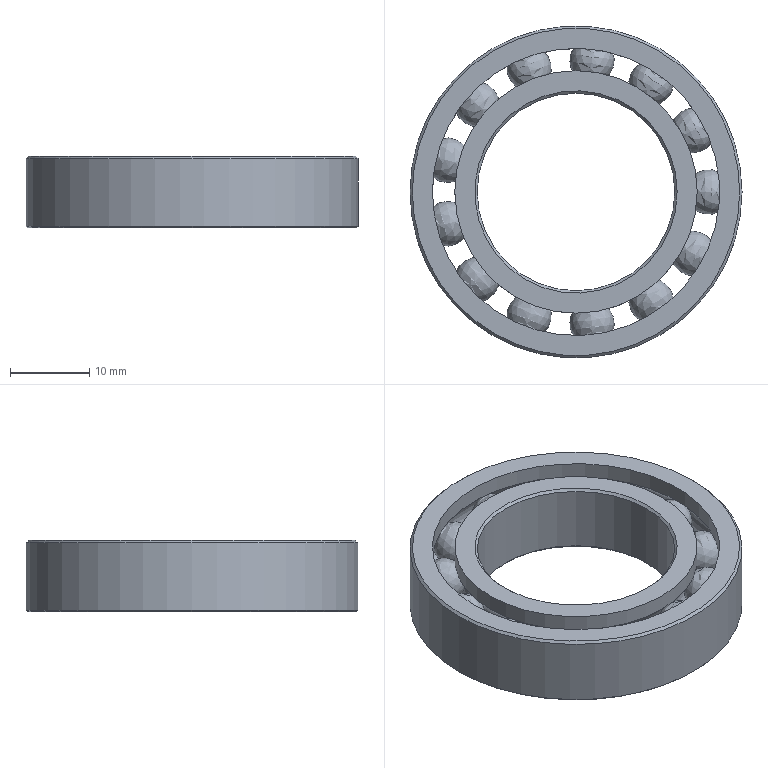Part | NX | features SWP104 18, INSTANCE_SET 12, CHAMFER 3, SKETCH 3, DATUM_CSYS 2, FSET 2, CIRCULAR_PATTERN 1, LINE 1 | 15 solids | 29 faces | box 42 x 42 x 9 mm | volume 5487 mm3 | sphere 13 | cylinder 5 | cone 5 | plane 4 | torus 2 | commonest cylinder face diameters 30.667 x2 25 x1 36.333 x1 42 x1
STEP:
#1=CARTESIAN_POINT('',(-13.513,3.331,4.5));
#2=VERTEX_POINT('',#1);
#3=VERTEX_LOOP('',#2);
#4=FACE_BOUND('',#3,.T.);
#5=CARTESIAN_POINT('',(-16.263,4.009,4.5));
#6=DIRECTION('',(-0.9709,0.2393,0.));
#7=DIRECTION('',(0.,0.,1.));
#8=AXIS2_PLACEMENT_3D('',#5,#6,#7);
#9=SPHERICAL_SURFACE('',#8,2.833);
#10=ADVANCED_FACE('',(#4),#9,.T.);
#11=CLOSED_SHELL('',(#10));
#12=MANIFOLD_SOLID_BREP('',#11);
#13=CARTESIAN_POINT('',(13.917,0.,4.5));
#14=VERTEX_POINT('',#13);
#15=VERTEX_LOOP('',#14);
#16=FACE_BOUND('',#15,.T.);
#17=CARTESIAN_POINT('',(16.75,0.,4.5));
#18=DIRECTION('',(1.,0.,0.));
#19=DIRECTION('',(0.,0.,1.));
#20=AXIS2_PLACEMENT_3D('',#17,#18,#19);
#21=SPHERICAL_SURFACE('',#20,2.833);
#22=ADVANCED_FACE('',(#16),#21,.T.);
#23=CLOSED_SHELL('',(#22));
#24=MANIFOLD_SOLID_BREP('',#23);
#25=CARTESIAN_POINT('',(7.906,11.454,4.5));
#26=VERTEX_POINT('',#25);
#27=VERTEX_LOOP('',#26);
#28=FACE_BOUND('',#27,.T.);
#29=CARTESIAN_POINT('',(9.515,13.785,4.5));
#30=DIRECTION('',(0.5681,0.823,0.));
#31=DIRECTION('',(0.,0.,1.));
#32=AXIS2_PLACEMENT_3D('',#29,#30,#31);
#33=SPHERICAL_SURFACE('',#32,2.833);
#34=ADVANCED_FACE('',(#28),#33,.T.);
#35=CLOSED_SHELL('',(#34));
#36=MANIFOLD_SOLID_BREP('',#35);
#37=CARTESIAN_POINT('',(1.678,-13.816,4.5));
#38=VERTEX_POINT('',#37);
#39=VERTEX_LOOP('',#38);
#40=FACE_BOUND('',#39,.T.);
#41=CARTESIAN_POINT('',(2.019,-16.628,4.5));
#42=DIRECTION('',(0.1205,-0.9927,0.));
#43=DIRECTION('',(0.,0.,1.));
#44=AXIS2_PLACEMENT_3D('',#41,#42,#43);
#45=SPHERICAL_SURFACE('',#44,2.833);
#46=ADVANCED_FACE('',(#40),#45,.T.);
#47=CLOSED_SHELL('',(#46));
#48=MANIFOLD_SOLID_BREP('',#47);
#49=CARTESIAN_POINT('',(1.678,13.816,4.5));
#50=VERTEX_POINT('',#49);
#51=VERTEX_LOOP('',#50);
#52=FACE_BOUND('',#51,.T.);
#53=CARTESIAN_POINT('',(2.019,16.628,4.5));
#54=DIRECTION('',(0.1205,0.9927,0.));
#55=DIRECTION('',(0.,0.,1.));
#56=AXIS2_PLACEMENT_3D('',#53,#54,#55);
#57=SPHERICAL_SURFACE('',#56,2.833);
#58=ADVANCED_FACE('',(#52),#57,.T.);
#59=CLOSED_SHELL('',(#58));
#60=MANIFOLD_SOLID_BREP('',#59);
#61=CARTESIAN_POINT('',(15.334,0.,2.047));
#62=VERTEX_POINT('',#61);
#63=CARTESIAN_POINT('',(0.,0.,2.047));
#64=DIRECTION('',(0.,0.,1.));
#65=DIRECTION('',(1.,0.,0.));
#66=AXIS2_PLACEMENT_3D('',#63,#64,#65);
#67=CIRCLE('',#66,15.334);
#68=EDGE_CURVE('',#62,#62,#67,.T.);
#69=ORIENTED_EDGE('',*,*,#68,.F.);
#70=EDGE_LOOP('',(#69));
#71=FACE_BOUND('',#70,.T.);
#72=CARTESIAN_POINT('',(-15.334,0.,0.));
#73=VERTEX_POINT('',#72);
#74=CARTESIAN_POINT('',(0.,0.,0.));
#75=DIRECTION('',(0.,0.,-1.));
#76=DIRECTION('',(-1.,0.,0.));
#77=AXIS2_PLACEMENT_3D('',#74,#75,#76);
#78=CIRCLE('',#77,15.334);
#79=EDGE_CURVE('',#73,#73,#78,.T.);
#80=ORIENTED_EDGE('',*,*,#79,.F.);
#81=EDGE_LOOP('',(#80));
#82=FACE_BOUND('',#81,.T.);
#83=CARTESIAN_POINT('',(0.,0.,0.));
#84=DIRECTION('',(0.,0.,-1.));
#85=DIRECTION('',(-1.,0.,0.));
#86=AXIS2_PLACEMENT_3D('',#83,#84,#85);
#87=CYLINDRICAL_SURFACE('',#86,15.334);
#88=ADVANCED_FACE('',(#71,#82),#87,.T.);
#89=CARTESIAN_POINT('',(-12.5,0.,0.3));
#90=VERTEX_POINT('',#89);
#91=CARTESIAN_POINT('',(0.,0.,0.3));
#92=DIRECTION('',(0.,0.,-1.));
#93=DIRECTION('',(-1.,0.,0.));
#94=AXIS2_PLACEMENT_3D('',#91,#92,#93);
#95=CIRCLE('',#94,12.5);
#96=EDGE_CURVE('',#90,#90,#95,.T.);
#97=ORIENTED_EDGE('',*,*,#96,.T.);
#98=EDGE_LOOP('',(#97));
#99=FACE_BOUND('',#98,.T.);
#100=CARTESIAN_POINT('',(12.5,0.,8.7));
#101=VERTEX_POINT('',#100);
#102=CARTESIAN_POINT('',(0.,0.,8.7));
#103=DIRECTION('',(0.,0.,1.));
#104=DIRECTION('',(1.,0.,0.));
#105=AXIS2_PLACEMENT_3D('',#102,#103,#104);
#106=CIRCLE('',#105,12.5);
#107=EDGE_CURVE('',#101,#101,#106,.T.);
#108=ORIENTED_EDGE('',*,*,#107,.T.);
#109=EDGE_LOOP('',(#108));
#110=FACE_BOUND('',#109,.T.);
#111=CARTESIAN_POINT('',(0.,0.,0.));
#112=DIRECTION('',(0.,0.,-1.));
#113=DIRECTION('',(-1.,0.,0.));
#114=AXIS2_PLACEMENT_3D('',#111,#112,#113);
#115=CYLINDRICAL_SURFACE('',#114,12.5);
#116=ADVANCED_FACE('',(#99,#110),#115,.F.);
#117=CARTESIAN_POINT('',(-12.8,0.,0.));
#118=VERTEX_POINT('',#117);
#119=CARTESIAN_POINT('',(0.,0.,0.));
#120=DIRECTION('',(0.,0.,-1.));
#121=DIRECTION('',(-1.,0.,0.));
#122=AXIS2_PLACEMENT_3D('',#119,#120,#121);
#123=CIRCLE('',#122,12.8);
#124=EDGE_CURVE('',#118,#118,#123,.F.);
#125=ORIENTED_EDGE('',*,*,#124,.T.);
#126=EDGE_LOOP('',(#125));
#127=FACE_BOUND('',#126,.T.);
#128=ORIENTED_EDGE('',*,*,#79,.T.);
#129=EDGE_LOOP('',(#128));
#130=FACE_BOUND('',#129,.T.);
#131=CARTESIAN_POINT('',(12.5,0.,0.));
#132=DIRECTION('',(0.,0.,-1.));
#133=DIRECTION('',(-1.,0.,0.));
#134=AXIS2_PLACEMENT_3D('',#131,#132,#133);
#135=PLANE('',#134);
#136=ADVANCED_FACE('',(#127,#130),#135,.T.);
#137=CARTESIAN_POINT('',(-15.334,0.,6.953));
#138=VERTEX_POINT('',#137);
#139=CARTESIAN_POINT('',(0.,0.,6.953));
#140=DIRECTION('',(0.,0.,-1.));
#141=DIRECTION('',(-1.,0.,0.));
#142=AXIS2_PLACEMENT_3D('',#139,#140,#141);
#143=CIRCLE('',#142,15.334);
#144=EDGE_CURVE('',#138,#138,#143,.T.);
#145=ORIENTED_EDGE('',*,*,#144,.F.);
#146=EDGE_LOOP('',(#145));
#147=FACE_BOUND('',#146,.T.);
#148=CARTESIAN_POINT('',(-15.334,0.,9.));
#149=VERTEX_POINT('',#148);
#150=CARTESIAN_POINT('',(0.,0.,9.));
#151=DIRECTION('',(0.,0.,-1.));
#152=DIRECTION('',(-1.,0.,0.));
#153=AXIS2_PLACEMENT_3D('',#150,#151,#152);
#154=CIRCLE('',#153,15.334);
#155=EDGE_CURVE('',#149,#149,#154,.T.);
#156=ORIENTED_EDGE('',*,*,#155,.T.);
#157=EDGE_LOOP('',(#156));
#158=FACE_BOUND('',#157,.T.);
#159=CARTESIAN_POINT('',(0.,0.,0.));
#160=DIRECTION('',(0.,0.,-1.));
#161=DIRECTION('',(-1.,0.,0.));
#162=AXIS2_PLACEMENT_3D('',#159,#160,#161);
#163=CYLINDRICAL_SURFACE('',#162,15.334);
#164=ADVANCED_FACE('',(#147,#158),#163,.T.);
#165=CARTESIAN_POINT('',(12.8,0.,9.));
#166=VERTEX_POINT('',#165);
#167=CARTESIAN_POINT('',(0.,0.,9.));
#168=DIRECTION('',(0.,0.,1.));
#169=DIRECTION('',(1.,0.,0.));
#170=AXIS2_PLACEMENT_3D('',#167,#168,#169);
#171=CIRCLE('',#170,12.8);
#172=EDGE_CURVE('',#166,#166,#171,.F.);
#173=ORIENTED_EDGE('',*,*,#172,.T.);
#174=EDGE_LOOP('',(#173));
#175=FACE_BOUND('',#174,.T.);
#176=ORIENTED_EDGE('',*,*,#155,.F.);
#177=EDGE_LOOP('',(#176));
#178=FACE_BOUND('',#177,.T.);
#179=CARTESIAN_POINT('',(15.334,0.,9.));
#180=DIRECTION('',(0.,0.,1.));
#181=DIRECTION('',(1.,0.,0.));
#182=AXIS2_PLACEMENT_3D('',#179,#180,#181);
#183=PLANE('',#182);
#184=ADVANCED_FACE('',(#175,#178),#183,.T.);
#185=ORIENTED_EDGE('',*,*,#68,.T.);
#186=EDGE_LOOP('',(#185));
#187=FACE_BOUND('',#186,.T.);
#188=ORIENTED_EDGE('',*,*,#144,.T.);
#189=EDGE_LOOP('',(#188));
#190=FACE_BOUND('',#189,.T.);
#191=CARTESIAN_POINT('',(0.,0.,4.5));
#192=DIRECTION('',(0.,0.,-1.));
#193=DIRECTION('',(-1.,0.,0.));
#194=AXIS2_PLACEMENT_3D('',#191,#192,#193);
#195=TOROIDAL_SURFACE('',#194,16.75,2.833);
#196=ADVANCED_FACE('',(#187,#190),#195,.F.);
#197=ORIENTED_EDGE('',*,*,#124,.F.);
#198=EDGE_LOOP('',(#197));
#199=FACE_BOUND('',#198,.T.);
#200=ORIENTED_EDGE('',*,*,#96,.F.);
#201=EDGE_LOOP('',(#200));
#202=FACE_BOUND('',#201,.T.);
#203=CARTESIAN_POINT('',(0.,0.,0.3));
#204=DIRECTION('',(0.,0.,-1.));
#205=DIRECTION('',(-1.,0.,0.));
#206=AXIS2_PLACEMENT_3D('',#203,#204,#205);
#207=CONICAL_SURFACE('',#206,12.5,0.7854);
#208=ADVANCED_FACE('',(#199,#202),#207,.F.);
#209=ORIENTED_EDGE('',*,*,#107,.F.);
#210=EDGE_LOOP('',(#209));
#211=FACE_BOUND('',#210,.T.);
#212=ORIENTED_EDGE('',*,*,#172,.F.);
#213=EDGE_LOOP('',(#212));
#214=FACE_BOUND('',#213,.T.);
#215=CARTESIAN_POINT('',(0.,0.,9.));
#216=DIRECTION('',(0.,0.,1.));
#217=DIRECTION('',(1.,0.,0.));
#218=AXIS2_PLACEMENT_3D('',#215,#216,#217);
#219=CONICAL_SURFACE('',#218,12.8,0.7854);
#220=ADVANCED_FACE('',(#211,#214),#219,.F.);
#221=CLOSED_SHELL('',(#88,#116,#136,#164,#184,#196,#208,#220));
#222=MANIFOLD_SOLID_BREP('',#221);
#223=CARTESIAN_POINT('',(-13.513,-3.331,4.5));
#224=VERTEX_POINT('',#223);
#225=VERTEX_LOOP('',#224);
#226=FACE_BOUND('',#225,.T.);
#227=CARTESIAN_POINT('',(-16.263,-4.009,4.5));
#228=DIRECTION('',(-0.9709,-0.2393,0.));
#229=DIRECTION('',(0.,0.,1.));
#230=AXIS2_PLACEMENT_3D('',#227,#228,#229);
#231=SPHERICAL_SURFACE('',#230,2.833);
#232=ADVANCED_FACE('',(#226),#231,.T.);
#233=CLOSED_SHELL('',(#232));
#234=MANIFOLD_SOLID_BREP('',#233);
#235=CARTESIAN_POINT('',(-21.,0.,0.15));
#236=VERTEX_POINT('',#235);
#237=CARTESIAN_POINT('',(0.,0.,0.15));
#238=DIRECTION('',(0.,0.,-1.));
#239=DIRECTION('',(-1.,0.,0.));
#240=AXIS2_PLACEMENT_3D('',#237,#238,#239);
#241=CIRCLE('',#240,21.);
#242=EDGE_CURVE('',#236,#236,#241,.F.);
#243=ORIENTED_EDGE('',*,*,#242,.T.);
#244=EDGE_LOOP('',(#243));
#245=FACE_BOUND('',#244,.T.);
#246=CARTESIAN_POINT('',(21.,0.,8.7));
#247=VERTEX_POINT('',#246);
#248=CARTESIAN_POINT('',(0.,0.,8.7));
#249=DIRECTION('',(0.,0.,1.));
#250=DIRECTION('',(1.,0.,0.));
#251=AXIS2_PLACEMENT_3D('',#248,#249,#250);
#252=CIRCLE('',#251,21.);
#253=EDGE_CURVE('',#247,#247,#252,.F.);
#254=ORIENTED_EDGE('',*,*,#253,.T.);
#255=EDGE_LOOP('',(#254));
#256=FACE_BOUND('',#255,.T.);
#257=CARTESIAN_POINT('',(0.,0.,0.));
#258=DIRECTION('',(0.,0.,-1.));
#259=DIRECTION('',(-1.,0.,0.));
#260=AXIS2_PLACEMENT_3D('',#257,#258,#259);
#261=CYLINDRICAL_SURFACE('',#260,21.);
#262=ADVANCED_FACE('',(#245,#256),#261,.T.);
#263=CARTESIAN_POINT('',(20.7,0.,9.));
#264=VERTEX_POINT('',#263);
#265=CARTESIAN_POINT('',(0.,0.,9.));
#266=DIRECTION('',(0.,0.,1.));
#267=DIRECTION('',(1.,0.,0.));
#268=AXIS2_PLACEMENT_3D('',#265,#266,#267);
#269=CIRCLE('',#268,20.7);
#270=EDGE_CURVE('',#264,#264,#269,.T.);
#271=ORIENTED_EDGE('',*,*,#270,.T.);
#272=EDGE_LOOP('',(#271));
#273=FACE_BOUND('',#272,.T.);
#274=CARTESIAN_POINT('',(-18.166,0.,9.));
#275=VERTEX_POINT('',#274);
#276=CARTESIAN_POINT('',(0.,0.,9.));
#277=DIRECTION('',(0.,0.,-1.));
#278=DIRECTION('',(-1.,0.,0.));
#279=AXIS2_PLACEMENT_3D('',#276,#277,#278);
#280=CIRCLE('',#279,18.166);
#281=EDGE_CURVE('',#275,#275,#280,.T.);
#282=ORIENTED_EDGE('',*,*,#281,.T.);
#283=EDGE_LOOP('',(#282));
#284=FACE_BOUND('',#283,.T.);
#285=CARTESIAN_POINT('',(21.,0.,9.));
#286=DIRECTION('',(0.,0.,1.));
#287=DIRECTION('',(1.,0.,0.));
#288=AXIS2_PLACEMENT_3D('',#285,#286,#287);
#289=PLANE('',#288);
#290=ADVANCED_FACE('',(#273,#284),#289,.T.);
#291=CARTESIAN_POINT('',(-18.166,0.,6.953));
#292=VERTEX_POINT('',#291);
#293=CARTESIAN_POINT('',(0.,0.,6.953));
#294=DIRECTION('',(0.,0.,-1.));
#295=DIRECTION('',(-1.,0.,0.));
#296=AXIS2_PLACEMENT_3D('',#293,#294,#295);
#297=CIRCLE('',#296,18.166);
#298=EDGE_CURVE('',#292,#292,#297,.F.);
#299=ORIENTED_EDGE('',*,*,#298,.F.);
#300=EDGE_LOOP('',(#299));
#301=FACE_BOUND('',#300,.T.);
#302=ORIENTED_EDGE('',*,*,#281,.F.);
#303=EDGE_LOOP('',(#302));
#304=FACE_BOUND('',#303,.T.);
#305=CARTESIAN_POINT('',(0.,0.,0.));
#306=DIRECTION('',(0.,0.,-1.));
#307=DIRECTION('',(-1.,0.,0.));
#308=AXIS2_PLACEMENT_3D('',#305,#306,#307);
#309=CYLINDRICAL_SURFACE('',#308,18.166);
#310=ADVANCED_FACE('',(#301,#304),#309,.F.);
#311=CARTESIAN_POINT('',(-20.85,0.,0.));
#312=VERTEX_POINT('',#311);
#313=CARTESIAN_POINT('',(0.,0.,0.));
#314=DIRECTION('',(0.,0.,-1.));
#315=DIRECTION('',(-1.,0.,0.));
#316=AXIS2_PLACEMENT_3D('',#313,#314,#315);
#317=CIRCLE('',#316,20.85);
#318=EDGE_CURVE('',#312,#312,#317,.T.);
#319=ORIENTED_EDGE('',*,*,#318,.T.);
#320=EDGE_LOOP('',(#319));
#321=FACE_BOUND('',#320,.T.);
#322=CARTESIAN_POINT('',(-18.733,0.,0.));
#323=VERTEX_POINT('',#322);
#324=CARTESIAN_POINT('',(0.,0.,0.));
#325=DIRECTION('',(0.,0.,-1.));
#326=DIRECTION('',(-1.,0.,0.));
#327=AXIS2_PLACEMENT_3D('',#324,#325,#326);
#328=CIRCLE('',#327,18.733);
#329=EDGE_CURVE('',#323,#323,#328,.T.);
#330=ORIENTED_EDGE('',*,*,#329,.F.);
#331=EDGE_LOOP('',(#330));
#332=FACE_BOUND('',#331,.T.);
#333=CARTESIAN_POINT('',(18.166,0.,0.));
#334=DIRECTION('',(0.,0.,-1.));
#335=DIRECTION('',(-1.,0.,0.));
#336=AXIS2_PLACEMENT_3D('',#333,#334,#335);
#337=PLANE('',#336);
#338=ADVANCED_FACE('',(#321,#332),#337,.T.);
#339=CARTESIAN_POINT('',(-18.166,0.,2.047));
#340=VERTEX_POINT('',#339);
#341=CARTESIAN_POINT('',(0.,0.,2.047));
#342=DIRECTION('',(0.,0.,-1.));
#343=DIRECTION('',(-1.,0.,0.));
#344=AXIS2_PLACEMENT_3D('',#341,#342,#343);
#345=CIRCLE('',#344,18.166);
#346=EDGE_CURVE('',#340,#340,#345,.T.);
#347=ORIENTED_EDGE('',*,*,#346,.T.);
#348=EDGE_LOOP('',(#347));
#349=FACE_BOUND('',#348,.T.);
#350=ORIENTED_EDGE('',*,*,#298,.T.);
#351=EDGE_LOOP('',(#350));
#352=FACE_BOUND('',#351,.T.);
#353=CARTESIAN_POINT('',(0.,0.,4.5));
#354=DIRECTION('',(0.,0.,-1.));
#355=DIRECTION('',(-1.,0.,0.));
#356=AXIS2_PLACEMENT_3D('',#353,#354,#355);
#357=TOROIDAL_SURFACE('',#356,16.75,2.833);
#358=ADVANCED_FACE('',(#349,#352),#357,.F.);
#359=ORIENTED_EDGE('',*,*,#346,.F.);
#360=EDGE_LOOP('',(#359));
#361=FACE_BOUND('',#360,.T.);
#362=ORIENTED_EDGE('',*,*,#329,.T.);
#363=EDGE_LOOP('',(#362));
#364=FACE_BOUND('',#363,.T.);
#365=CARTESIAN_POINT('',(0.,0.,0.));
#366=DIRECTION('',(0.,0.,-1.));
#367=DIRECTION('',(-1.,0.,0.));
#368=AXIS2_PLACEMENT_3D('',#365,#366,#367);
#369=CONICAL_SURFACE('',#368,18.733,0.2701);
#370=ADVANCED_FACE('',(#361,#364),#369,.F.);
#371=ORIENTED_EDGE('',*,*,#270,.F.);
#372=EDGE_LOOP('',(#371));
#373=FACE_BOUND('',#372,.T.);
#374=ORIENTED_EDGE('',*,*,#253,.F.);
#375=EDGE_LOOP('',(#374));
#376=FACE_BOUND('',#375,.T.);
#377=CARTESIAN_POINT('',(0.,0.,8.7));
#378=DIRECTION('',(0.,0.,-1.));
#379=DIRECTION('',(-1.,0.,0.));
#380=AXIS2_PLACEMENT_3D('',#377,#378,#379);
#381=CONICAL_SURFACE('',#380,21.,0.7854);
#382=ADVANCED_FACE('',(#373,#376),#381,.T.);
#383=ORIENTED_EDGE('',*,*,#242,.F.);
#384=EDGE_LOOP('',(#383));
#385=FACE_BOUND('',#384,.T.);
#386=ORIENTED_EDGE('',*,*,#318,.F.);
#387=EDGE_LOOP('',(#386));
#388=FACE_BOUND('',#387,.T.);
#389=CARTESIAN_POINT('',(0.,0.,0.));
#390=DIRECTION('',(0.,0.,1.));
#391=DIRECTION('',(1.,0.,0.));
#392=AXIS2_PLACEMENT_3D('',#389,#390,#391);
#393=CONICAL_SURFACE('',#392,20.85,0.7854);
#394=ADVANCED_FACE('',(#385,#388),#393,.T.);
#395=CLOSED_SHELL('',(#262,#290,#310,#338,#358,#370,#382,#394));
#396=MANIFOLD_SOLID_BREP('',#395);
#397=CARTESIAN_POINT('',(12.323,-6.468,4.5));
#398=VERTEX_POINT('',#397);
#399=VERTEX_LOOP('',#398);
#400=FACE_BOUND('',#399,.T.);
#401=CARTESIAN_POINT('',(14.831,-7.784,4.5));
#402=DIRECTION('',(0.8855,-0.4647,0.));
#403=DIRECTION('',(0.,0.,1.));
#404=AXIS2_PLACEMENT_3D('',#401,#402,#403);
#405=SPHERICAL_SURFACE('',#404,2.833);
#406=ADVANCED_FACE('',(#400),#405,.T.);
#407=CLOSED_SHELL('',(#406));
#408=MANIFOLD_SOLID_BREP('',#407);
#409=CARTESIAN_POINT('',(12.323,6.468,4.5));
#410=VERTEX_POINT('',#409);
#411=VERTEX_LOOP('',#410);
#412=FACE_BOUND('',#411,.T.);
#413=CARTESIAN_POINT('',(14.831,7.784,4.5));
#414=DIRECTION('',(0.8855,0.4647,0.));
#415=DIRECTION('',(0.,0.,1.));
#416=AXIS2_PLACEMENT_3D('',#413,#414,#415);
#417=SPHERICAL_SURFACE('',#416,2.833);
#418=ADVANCED_FACE('',(#412),#417,.T.);
#419=CLOSED_SHELL('',(#418));
#420=MANIFOLD_SOLID_BREP('',#419);
#421=CARTESIAN_POINT('',(-10.417,-9.229,4.5));
#422=VERTEX_POINT('',#421);
#423=VERTEX_LOOP('',#422);
#424=FACE_BOUND('',#423,.T.);
#425=CARTESIAN_POINT('',(-12.538,-11.107,4.5));
#426=DIRECTION('',(-0.7485,-0.6631,0.));
#427=DIRECTION('',(0.,0.,1.));
#428=AXIS2_PLACEMENT_3D('',#425,#426,#427);
#429=SPHERICAL_SURFACE('',#428,2.833);
#430=ADVANCED_FACE('',(#424),#429,.T.);
#431=CLOSED_SHELL('',(#430));
#432=MANIFOLD_SOLID_BREP('',#431);
#433=CARTESIAN_POINT('',(-4.935,13.013,4.5));
#434=VERTEX_POINT('',#433);
#435=VERTEX_LOOP('',#434);
#436=FACE_BOUND('',#435,.T.);
#437=CARTESIAN_POINT('',(-5.94,15.662,4.5));
#438=DIRECTION('',(-0.3546,0.935,0.));
#439=DIRECTION('',(0.,0.,1.));
#440=AXIS2_PLACEMENT_3D('',#437,#438,#439);
#441=SPHERICAL_SURFACE('',#440,2.833);
#442=ADVANCED_FACE('',(#436),#441,.T.);
#443=CLOSED_SHELL('',(#442));
#444=MANIFOLD_SOLID_BREP('',#443);
#445=CARTESIAN_POINT('',(-10.417,9.229,4.5));
#446=VERTEX_POINT('',#445);
#447=VERTEX_LOOP('',#446);
#448=FACE_BOUND('',#447,.T.);
#449=CARTESIAN_POINT('',(-12.538,11.107,4.5));
#450=DIRECTION('',(-0.7485,0.6631,0.));
#451=DIRECTION('',(0.,0.,1.));
#452=AXIS2_PLACEMENT_3D('',#449,#450,#451);
#453=SPHERICAL_SURFACE('',#452,2.833);
#454=ADVANCED_FACE('',(#448),#453,.T.);
#455=CLOSED_SHELL('',(#454));
#456=MANIFOLD_SOLID_BREP('',#455);
#457=CARTESIAN_POINT('',(7.906,-11.454,4.5));
#458=VERTEX_POINT('',#457);
#459=VERTEX_LOOP('',#458);
#460=FACE_BOUND('',#459,.T.);
#461=CARTESIAN_POINT('',(9.515,-13.785,4.5));
#462=DIRECTION('',(0.5681,-0.823,0.));
#463=DIRECTION('',(0.,0.,1.));
#464=AXIS2_PLACEMENT_3D('',#461,#462,#463);
#465=SPHERICAL_SURFACE('',#464,2.833);
#466=ADVANCED_FACE('',(#460),#465,.T.);
#467=CLOSED_SHELL('',(#466));
#468=MANIFOLD_SOLID_BREP('',#467);
#469=CARTESIAN_POINT('',(-4.935,-13.013,4.5));
#470=VERTEX_POINT('',#469);
#471=VERTEX_LOOP('',#470);
#472=FACE_BOUND('',#471,.T.);
#473=CARTESIAN_POINT('',(-5.94,-15.662,4.5));
#474=DIRECTION('',(-0.3546,-0.935,0.));
#475=DIRECTION('',(0.,0.,1.));
#476=AXIS2_PLACEMENT_3D('',#473,#474,#475);
#477=SPHERICAL_SURFACE('',#476,2.833);
#478=ADVANCED_FACE('',(#472),#477,.T.);
#479=CLOSED_SHELL('',(#478));
#480=MANIFOLD_SOLID_BREP('',#479);
#481=(LENGTH_UNIT()NAMED_UNIT(*)SI_UNIT(.MILLI.,.METRE.));
#482=UNCERTAINTY_MEASURE_WITH_UNIT(LENGTH_MEASURE(0.00001),#481,'','');
#483=(NAMED_UNIT(*)PLANE_ANGLE_UNIT()SI_UNIT($,.RADIAN.));
#484=(NAMED_UNIT(*)SI_UNIT($,.STERADIAN.)SOLID_ANGLE_UNIT());
#485=(GEOMETRIC_REPRESENTATION_CONTEXT(3)GLOBAL_UNCERTAINTY_ASSIGNED_CONTEXT((#482))GLOBAL_UNIT_ASSIGNED_CONTEXT((#481,#483,#484))REPRESENTATION_CONTEXT('',''));
#486=ADVANCED_BREP_SHAPE_REPRESENTATION('',(#12,#24,#36,#48,#60,#222,#234,#396,#408,#420,#432,#444,#456,#468,#480),#485);